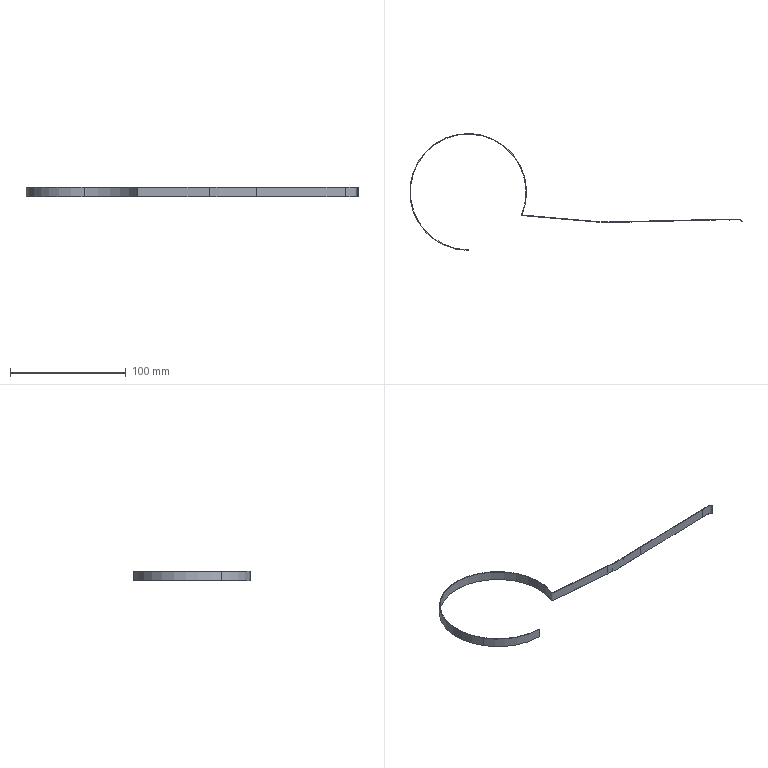Part | NX | features BREP 2, Delete Body 2, LINKED_FACE 2, SPLIT BODY 2, DATUM_PLANE 1 | 5 solids | 30 faces | box 287.083 x 101 x 8 mm | volume 631.847 mm3 | plane 20 | spline 8 | cylinder 2 | commonest cylinder face diameters 3.18 x1 4.18 x1